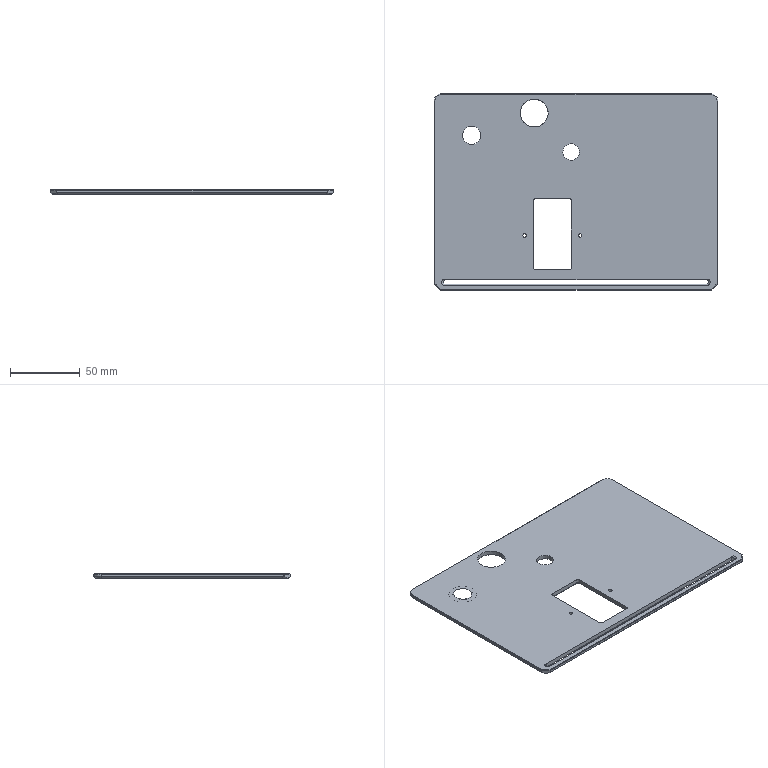Part | SolidWorks | features BaseBody 1 | 1 solid | 970 faces | box 204 x 141.5 x 3.5 mm | volume 90063 mm3 | plane 535 | spline 382 | cone 32 | cylinder 21 | commonest cylinder face diameters 1 x4 2.5 x4 3 x4 3.1 x3 11 x2 12 x2